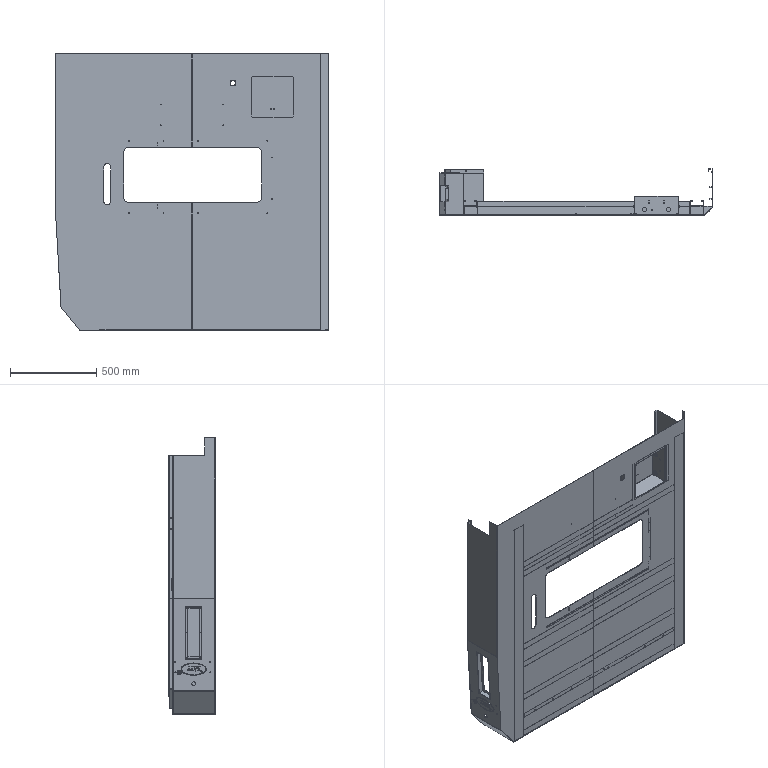Part | SolidWorks | 25 solids | 1461 faces | box 1580 x 269 x 1600 mm | volume 11681636 mm3 | plane 812 | cylinder 603 | spline 42 | cone 4 | commonest cylinder face diameters 4.2 x104 6 x95 0.4 x62 3.3 x58 3 x48 3.4 x36